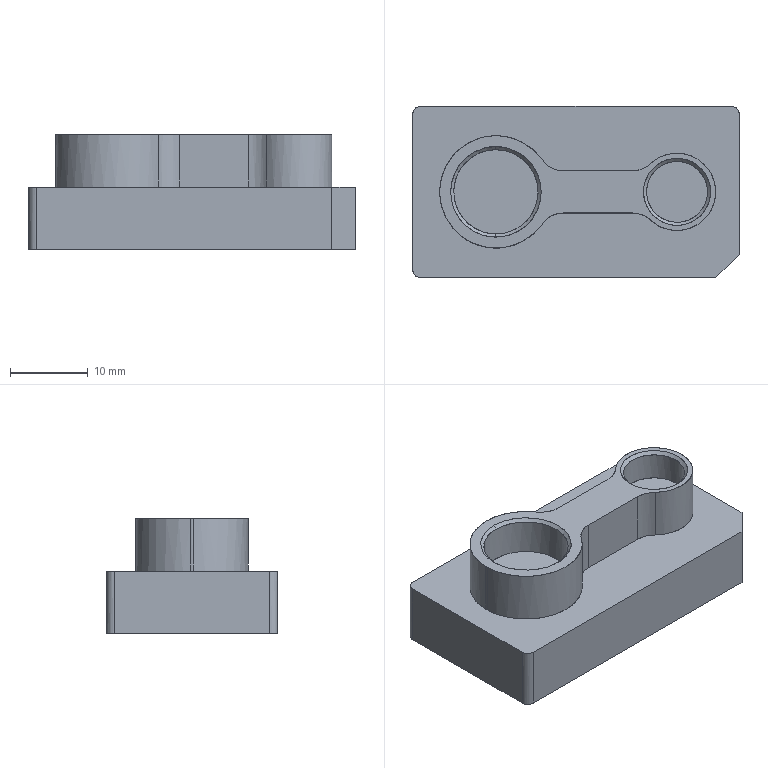NC program | PowerMill | posted by the shop | part box 42 x 22 x 14.721 mm
Lines 13163 to 14231 of 84704:
( TOOL ID   R1_1 )
( TOOL DIA. 2. TIP RAD 1. LENGTH 57. )
( Z = -1.104 )
T4 M6
T14
G91 G28 Z0
G0 G90 G54
M08
S18000 M3
X0 Y0 M8
G43 Z10.801 H4
X15.909 Y-2.486
Z.787
G1 Z-.413 F1200
X15.867 Y-2.527 Z-.416 F2000
X15.764 Y-2.63 Z-.42
X15.658 Y-2.737 Z-.421
X15.555 Y-2.84 Z-.418
X15.451 Y-2.943 Z-.411
X15.264 Y-3.088 Z-.412
X15.363 Y-2.989 Z-.424
X15.462 Y-2.89 Z-.433
X15.561 Y-2.791 Z-.439
X15.66 Y-2.692 Z-.441
X15.762 Y-2.59 Z-.44
X15.861 Y-2.491 Z-.435
X15.96 Y-2.392 Z-.427
X16.059 Y-2.293 Z-.416
X16.096 Y-2.256 Z-.411
X16.179 Y-2.13 Z-.413
X16.099 Y-2.211 Z-.426
X16.008 Y-2.301 Z-.439
X15.917 Y-2.392 Z-.45
X15.821 Y-2.489 Z-.458
X15.723 Y-2.587 Z-.463
X15.632 Y-2.678 Z-.464
X15.541 Y-2.769 Z-.461
X15.45 Y-2.86 Z-.455
X15.359 Y-2.95 Z-.446
X15.257 Y-3.053 Z-.433
X15.135 Y-3.174 Z-.414
X15.02 Y-3.247 Z-.415
X15.104 Y-3.163 Z-.431
X15.189 Y-3.078 Z-.447
X15.276 Y-2.991 Z-.461
X15.372 Y-2.895 Z-.473
X15.466 Y-2.801 Z-.482
X15.551 Y-2.717 Z-.486
X15.636 Y-2.632 Z-.488
X15.721 Y-2.547 Z-.486
X15.805 Y-2.462 Z-.481
X15.901 Y-2.366 Z-.472
X16.004 Y-2.263 Z-.459
X16.117 Y-2.15 Z-.44
X16.239 Y-2.028 Z-.416
X16.299 Y-1.926 Z-.418
X16.275 Y-1.949 Z-.423
X16.142 Y-2.083 Z-.452
X16.028 Y-2.197 Z-.474
X15.925 Y-2.3 Z-.491
X15.83 Y-2.394 Z-.503
X15.749 Y-2.476 Z-.51
X15.667 Y-2.558 Z-.514
X15.585 Y-2.64
X15.502 Y-2.723 Z-.511
X15.42 Y-2.804 Z-.505
X15.339 Y-2.886 Z-.496
X15.257 Y-2.967 Z-.485
X15.171 Y-3.053 Z-.47
X15.086 Y-3.139 Z-.453
X15. Y-3.225 Z-.434
X14.914 Y-3.31 Z-.415
X14.818 Y-3.365
X14.936 Y-3.246 Z-.445
X15.061 Y-3.121 Z-.475
X15.171 Y-3.011 Z-.498
X15.27 Y-2.912 Z-.516
X15.361 Y-2.821 Z-.529
X15.445 Y-2.737 Z-.537
X15.53 Y-2.652 Z-.542
X15.614 Y-2.568 Z-.543
X15.698 Y-2.484 Z-.54
X15.782 Y-2.401 Z-.533
X15.869 Y-2.313 Z-.523
X15.965 Y-2.218 Z-.507
X16.069 Y-2.113 Z-.486
X16.185 Y-1.998 Z-.46
X16.296 Y-1.886 Z-.432
X16.354 Y-1.828 Z-.417
X16.405 Y-1.735
X16.329 Y-1.811 Z-.438
X16.249 Y-1.891 Z-.46
X16.169 Y-1.971 Z-.482
X16.084 Y-2.056 Z-.504
X15.992 Y-2.148 Z-.525
X15.899 Y-2.241 Z-.543
X15.814 Y-2.326 Z-.557
X15.735 Y-2.404 Z-.566
X15.658 Y-2.482 Z-.571
X15.581 Y-2.559 Z-.573
X15.503 Y-2.637 Z-.572
X15.425 Y-2.714 Z-.567
X15.348 Y-2.792 Z-.56
X15.266 Y-2.873 Z-.548
X15.189 Y-2.951 Z-.534
X15.113 Y-3.027 Z-.517
X15.036 Y-3.104 Z-.499
X14.908 Y-3.232 Z-.465
X14.725 Y-3.415 Z-.414
X14.644 Y-3.453 Z-.415
X14.817 Y-3.28 Z-.467
X14.888 Y-3.209 Z-.489
X14.96 Y-3.138 Z-.51
X15.031 Y-3.066 Z-.53
X15.109 Y-2.988 Z-.55
X15.196 Y-2.902 Z-.569
X15.275 Y-2.822 Z-.583
X15.348 Y-2.75 Z-.592
X15.421 Y-2.677 Z-.599
X15.493 Y-2.604 Z-.602
X15.566 Y-2.531 Z-.603
X15.639 Y-2.458 Z-.601
X15.719 Y-2.378 Z-.595
X15.803 Y-2.295 Z-.585
X15.888 Y-2.209 Z-.571
X15.97 Y-2.127 Z-.554
X16.049 Y-2.048 Z-.534
X16.149 Y-1.948 Z-.507
X16.249 Y-1.848 Z-.477
X16.349 Y-1.749 Z-.446
X16.449 Y-1.649 Z-.416
Y-1.648
X16.485 Y-1.57
X16.449 Y-1.606 Z-.428
X16.389 Y-1.666 Z-.447
X16.329 Y-1.726 Z-.467
X16.27 Y-1.785 Z-.487
X16.21 Y-1.845 Z-.507
X16.15 Y-1.905 Z-.527
X16.09 Y-1.965 Z-.546
X16.023 Y-2.032 Z-.565
X15.959 Y-2.096 Z-.582
X15.898 Y-2.157 Z-.595
X15.837 Y-2.218 Z-.606
X15.776 Y-2.279 Z-.616
X15.702 Y-2.353 Z-.625
X15.618 Y-2.437 Z-.631
X15.533 Y-2.522 Z-.633
X15.449 Y-2.606 Z-.631
X15.364 Y-2.691 Z-.626
X15.279 Y-2.776 Z-.616
X15.199 Y-2.856 Z-.603
X15.117 Y-2.938 Z-.586
X15.029 Y-3.026 Z-.564
X14.933 Y-3.122 Z-.536
X14.855 Y-3.2 Z-.511
X14.71 Y-3.345 Z-.462
X14.565 Y-3.49 Z-.414
X14.492 Y-3.52 Z-.415
X14.704 Y-3.309 Z-.491
X14.796 Y-3.217 Z-.524
X14.891 Y-3.122 Z-.558
X14.982 Y-3.03 Z-.586
X15.07 Y-2.943 Z-.61
X15.155 Y-2.857 Z-.629
X15.238 Y-2.775 Z-.643
X15.321 Y-2.692 Z-.654
X15.404 Y-2.608 Z-.66
X15.489 Y-2.524 Z-.663
X15.573 Y-2.439 Z-.662
X15.659 Y-2.354 Z-.656
X15.744 Y-2.268 Z-.647
X15.83 Y-2.182 Z-.634
X15.916 Y-2.096 Z-.617
X15.972 Y-2.041 Z-.603
X16.027 Y-1.986 Z-.587
X16.082 Y-1.931 Z-.57
X16.137 Y-1.876 Z-.553
X16.192 Y-1.821 Z-.534
X16.246 Y-1.766 Z-.513
X16.426 Y-1.587 Z-.448
X16.519 Y-1.493 Z-.415
X16.549 Y-1.421 Z-.416
X16.467 Y-1.503 Z-.445
X16.349 Y-1.621 Z-.491
X16.246 Y-1.724 Z-.532
X16.166 Y-1.804 Z-.564
X16.086 Y-1.884 Z-.592
X16.003 Y-1.968 Z-.618
X15.916 Y-2.054 Z-.641
X15.834 Y-2.136 Z-.659
X15.752 Y-2.218 Z-.673
X15.67 Y-2.301 Z-.684
X15.585 Y-2.385 Z-.69
X15.501 Y-2.47 Z-.693
X15.416 Y-2.554 Z-.692
X15.332 Y-2.638 Z-.687
X15.248 Y-2.722 Z-.677
X15.164 Y-2.806 Z-.664
X15.08 Y-2.891 Z-.647
X14.994 Y-2.976 Z-.625
X14.909 Y-3.062 Z-.6
X14.822 Y-3.148 Z-.57
X14.74 Y-3.23 Z-.538
X14.635 Y-3.335 Z-.497
X14.529 Y-3.441 Z-.455
X14.423 Y-3.547 Z-.416
X14.353 Y-3.574
X14.441 Y-3.487 Z-.45
X14.538 Y-3.39 Z-.489
X14.653 Y-3.275 Z-.539
X14.741 Y-3.187 Z-.576
X14.829 Y-3.099 Z-.609
X14.916 Y-3.012 Z-.638
X15.004 Y-2.924 Z-.663
X15.087 Y-2.841 Z-.683
X15.171 Y-2.757 Z-.699
X15.255 Y-2.673 Z-.711
X15.339 Y-2.589 Z-.719
X15.422 Y-2.505 Z-.723
X15.506 Y-2.422
X15.589 Y-2.339 Z-.719
X15.671 Y-2.257 Z-.711
X15.754 Y-2.174 Z-.699
X15.834 Y-2.094 Z-.684
X15.899 Y-2.029 Z-.669
X15.964 Y-1.964 Z-.652
X16.028 Y-1.9 Z-.633
X16.092 Y-1.836 Z-.612
X16.156 Y-1.772 Z-.588
X16.219 Y-1.709 Z-.563
X16.282 Y-1.646 Z-.536
X16.345 Y-1.583 Z-.509
X16.408 Y-1.519 Z-.482
X16.472 Y-1.456 Z-.456
X16.535 Y-1.393 Z-.431
X16.578 Y-1.35 Z-.415
X16.601 Y-1.285 Z-.416
X16.577 Y-1.308 Z-.425
X16.477 Y-1.408 Z-.466
X16.428 Y-1.457 Z-.487
X16.379 Y-1.506 Z-.51
X16.313 Y-1.572 Z-.54
X16.264 Y-1.621 Z-.563
X16.215 Y-1.67 Z-.585
X16.166 Y-1.719 Z-.606
X16.095 Y-1.791 Z-.632
X16.019 Y-1.866 Z-.658
X15.934 Y-1.952 Z-.684
X15.857 Y-2.028 Z-.704
X15.781 Y-2.105 Z-.72
X15.701 Y-2.185 Z-.734
X15.618 Y-2.268 Z-.744
X15.534 Y-2.352 Z-.751
X15.453 Y-2.433 Z-.753
X15.372 Y-2.513 Z-.752
X15.289 Y-2.596 Z-.746
X15.206 Y-2.68 Z-.737
X15.122 Y-2.764 Z-.724
X15.037 Y-2.848 Z-.706
X14.953 Y-2.933 Z-.685
X14.868 Y-3.018 Z-.659
X14.782 Y-3.103 Z-.629
X14.699 Y-3.186 Z-.597
X14.623 Y-3.262 Z-.564
X14.529 Y-3.356 Z-.52
X14.442 Y-3.444 Z-.481
X14.352 Y-3.533 Z-.442
X14.288 Y-3.598 Z-.417
X14.223 Y-3.619
X14.282 Y-3.561 Z-.441
X14.34 Y-3.503 Z-.467
X14.398 Y-3.445 Z-.494
X14.456 Y-3.387 Z-.521
X14.529 Y-3.314 Z-.558
X14.602 Y-3.241 Z-.592
X14.689 Y-3.154 Z-.63
X14.779 Y-3.064 Z-.664
X14.87 Y-2.973 Z-.696
X14.948 Y-2.895 Z-.718
X15.028 Y-2.815 Z-.738
X15.112 Y-2.731 Z-.755
X15.196 Y-2.646 Z-.768
X15.278 Y-2.564 Z-.777
X15.358 Y-2.485 Z-.782
X15.437 Y-2.406 Z-.783
X15.519 Y-2.324 Z-.78
X15.602 Y-2.241 Z-.774
X15.685 Y-2.158 Z-.763
X15.769 Y-2.074 Z-.748
X15.854 Y-1.989 Z-.729
X15.939 Y-1.904 Z-.706
X16.025 Y-1.818 Z-.678
X16.111 Y-1.732 Z-.647
X16.188 Y-1.655 Z-.616
X16.256 Y-1.587 Z-.585
X16.337 Y-1.506 Z-.545
X16.398 Y-1.445 Z-.516
X16.462 Y-1.381 Z-.486
X16.52 Y-1.323 Z-.459
X16.586 Y-1.257 Z-.432
X16.621 Y-1.222 Z-.417
X16.641 Y-1.16
X16.598 Y-1.203 Z-.435
X16.504 Y-1.297 Z-.478
X16.414 Y-1.386 Z-.523
X16.325 Y-1.475 Z-.57
X16.244 Y-1.556 Z-.61
X16.156 Y-1.644 Z-.649
X16.068 Y-1.733 Z-.684
X15.981 Y-1.819 Z-.715
X15.896 Y-1.905 Z-.742
X15.811 Y-1.989 Z-.764
X15.727 Y-2.073 Z-.782
X15.644 Y-2.157 Z-.796
X15.561 Y-2.239 Z-.806
X15.48 Y-2.321 Z-.811
X15.399 Y-2.401 Z-.813
X15.317 Y-2.483 Z-.811
X15.235 Y-2.565 Z-.805
X15.153 Y-2.648 Z-.795
X15.07 Y-2.73 Z-.781
X14.987 Y-2.813 Z-.763
X14.903 Y-2.897 Z-.741
X14.819 Y-2.981 Z-.715
X14.735 Y-3.066 Z-.685
X14.656 Y-3.145 Z-.654
X14.583 Y-3.218 Z-.621
X14.508 Y-3.292 Z-.585
X14.442 Y-3.359 Z-.553
X14.372 Y-3.428 Z-.517
X14.297 Y-3.504 Z-.479
X14.24 Y-3.56 Z-.452
X14.161 Y-3.64 Z-.417
X14.099 Y-3.659
X14.163 Y-3.595 Z-.446
X14.225 Y-3.533 Z-.476
X14.288 Y-3.47 Z-.508
X14.354 Y-3.404 Z-.544
X14.418 Y-3.341 Z-.578
X14.481 Y-3.277 Z-.612
X14.57 Y-3.188 Z-.654
X14.652 Y-3.106 Z-.69
X14.741 Y-3.017 Z-.724
X14.827 Y-2.931 Z-.754
X14.91 Y-2.848 Z-.778
X14.993 Y-2.765 Z-.799
X15.077 Y-2.681 Z-.816
X15.16 Y-2.598 Z-.829
X15.243 Y-2.515 Z-.838
X15.322 Y-2.436 Z-.842
X15.4 Y-2.358 Z-.843
X15.482 Y-2.276 Z-.84
X15.565 Y-2.193 Z-.832
X15.648 Y-2.11 Z-.821
X15.728 Y-2.03 Z-.807
X15.798 Y-1.96 Z-.791
X15.872 Y-1.886 Z-.771
X15.966 Y-1.792 Z-.742
X15.999 Y-1.759 Z-.731
X16.032 Y-1.726 Z-.719
X16.065 Y-1.694 Z-.706
X16.097 Y-1.661 Z-.693
X16.14 Y-1.618 Z-.675
X16.173 Y-1.585 Z-.661
X16.205 Y-1.553 Z-.646
X16.237 Y-1.521 Z-.631
X16.269 Y-1.489 Z-.615
X16.354 Y-1.404 Z-.571
X16.436 Y-1.322 Z-.527
X16.508 Y-1.25 Z-.488
X16.568 Y-1.19 Z-.458
X16.635 Y-1.123 Z-.428
X16.66 Y-1.098 Z-.417
X16.68 Y-1.036 Z-.416
X16.64 Y-1.076 Z-.434
X16.58 Y-1.136 Z-.463
X16.524 Y-1.192 Z-.492
X16.46 Y-1.255 Z-.529
X16.392 Y-1.324 Z-.566
X16.295 Y-1.421 Z-.619
X16.228 Y-1.487 Z-.653
X16.139 Y-1.577 Z-.695
X16.051 Y-1.665 Z-.732
X15.964 Y-1.752 Z-.765
X15.879 Y-1.837 Z-.793
X15.795 Y-1.92 Z-.816
X15.712 Y-2.003 Z-.836
X15.63 Y-2.086 Z-.851
X15.548 Y-2.168 Z-.862
X15.466 Y-2.249 Z-.87
X15.385 Y-2.331 Z-.873
X15.304 Y-2.412 Z-.872
X15.223 Y-2.493 Z-.868
X15.142 Y-2.574 Z-.859
X15.06 Y-2.655 Z-.847
X14.978 Y-2.738 Z-.83
X14.894 Y-2.822 Z-.809
X14.809 Y-2.906 Z-.784
X14.723 Y-2.992 Z-.755
X14.637 Y-3.079 Z-.721
X14.561 Y-3.155 Z-.688
X14.477 Y-3.239 Z-.647
X14.371 Y-3.345 Z-.592
X14.328 Y-3.388 Z-.569
X14.277 Y-3.439 Z-.539
X14.234 Y-3.481 Z-.515
X14.156 Y-3.559 Z-.474
X14.092 Y-3.624 Z-.441
X14.039 Y-3.677 Z-.417
X13.978 Y-3.695 Z-.416
X14.014 Y-3.659 Z-.433
X14.05 Y-3.623 Z-.45
X14.086 Y-3.587 Z-.469
X14.159 Y-3.514 Z-.51
X14.242 Y-3.431 Z-.559
X14.325 Y-3.348 Z-.606
X14.393 Y-3.28 Z-.644
X14.462 Y-3.211 Z-.679
X14.551 Y-3.122 Z-.722
X14.638 Y-3.035 Z-.759
X14.723 Y-2.95 Z-.791
X14.808 Y-2.865 Z-.82
X14.892 Y-2.781 Z-.844
X14.975 Y-2.699 Z-.864
X15.057 Y-2.616 Z-.88
X15.139 Y-2.535 Z-.891
X15.22 Y-2.454 Z-.899
X15.3 Y-2.373 Z-.903
X15.355 Y-2.318
X15.41 Y-2.263 Z-.901
X15.465 Y-2.208 Z-.898
X15.52 Y-2.153 Z-.892
X15.575 Y-2.099 Z-.886
X15.629 Y-2.044 Z-.877
X15.715 Y-1.958 Z-.86
X15.801 Y-1.872 Z-.839
X15.886 Y-1.788 Z-.813
X15.969 Y-1.704 Z-.784
X16.053 Y-1.621 Z-.752
X16.141 Y-1.532 Z-.713
X16.233 Y-1.44 Z-.669
X16.292 Y-1.381 Z-.637
X16.351 Y-1.322 Z-.604
X16.41 Y-1.263 Z-.57
X16.459 Y-1.215 Z-.542
X16.518 Y-1.155 Z-.507
X16.566 Y-1.107 Z-.48
X16.622 Y-1.051 Z-.451
X16.679 Y-.994 Z-.423
X16.699 Y-.974 Z-.415
X16.713 Y-.917
X16.7 Y-.931 Z-.421
X16.643 Y-.987 Z-.448
X16.605 Y-1.026 Z-.469
X16.528 Y-1.103 Z-.513
X16.495 Y-1.136 Z-.533
X16.461 Y-1.17 Z-.553
X16.428 Y-1.203 Z-.574
X16.394 Y-1.236 Z-.594
X16.361 Y-1.27 Z-.615
X16.327 Y-1.304 Z-.634
X16.235 Y-1.396 Z-.685
X16.142 Y-1.489 Z-.731
X16.054 Y-1.577 Z-.771
X15.967 Y-1.664 Z-.806
X15.882 Y-1.749 Z-.837
X15.797 Y-1.833 Z-.863
X15.714 Y-1.917 Z-.885
X15.632 Y-1.999 Z-.903
X15.551 Y-2.08 Z-.916
X15.471 Y-2.16 Z-.926
X15.391 Y-2.24 Z-.931
X15.309 Y-2.321 Z-.933
X15.23 Y-2.4 Z-.931
X15.151 Y-2.48 Z-.925
X15.071 Y-2.56 Z-.915
X14.989 Y-2.642 Z-.901
X14.906 Y-2.724 Z-.882
X14.823 Y-2.808 Z-.86
X14.738 Y-2.892 Z-.833
X14.653 Y-2.978 Z-.802
X14.567 Y-3.064 Z-.766
X14.475 Y-3.155 Z-.724
X14.385 Y-3.246 Z-.679
X14.29 Y-3.341 Z-.626
X14.196 Y-3.435 Z-.57
X14.141 Y-3.49 Z-.536
X14.074 Y-3.556 Z-.496
X14.021 Y-3.61 Z-.466
X13.962 Y-3.668 Z-.436
X13.92 Y-3.711 Z-.416
X13.862 Y-3.726 Z-.415
X13.882 Y-3.707 Z-.424
X13.901 Y-3.687 Z-.434
X13.928 Y-3.661 Z-.447
X13.947 Y-3.641 Z-.458
X13.966 Y-3.622 Z-.468
X13.985 Y-3.603 Z-.479
X14.044 Y-3.545 Z-.515
X14.098 Y-3.49 Z-.549
X14.178 Y-3.41 Z-.599
X14.252 Y-3.336 Z-.644
X14.344 Y-3.244 Z-.696
X14.436 Y-3.152 Z-.744
X14.524 Y-3.064 Z-.785
X14.611 Y-2.977 Z-.823
X14.698 Y-2.89 Z-.856
X14.774 Y-2.814 Z-.881
X14.852 Y-2.736 Z-.903
X14.933 Y-2.655 Z-.923
X15.016 Y-2.572 Z-.94
X15.099 Y-2.49 Z-.952
X15.179 Y-2.409 Z-.96
X15.257 Y-2.331 Z-.964
X15.331 Y-2.257
X15.403 Y-2.185 Z-.961
X15.475 Y-2.113 Z-.954
X15.559 Y-2.03 Z-.942
X15.642 Y-1.946 Z-.926
X15.726 Y-1.862 Z-.906
X15.81 Y-1.778 Z-.882
X15.894 Y-1.694 Z-.854
X15.978 Y-1.61 Z-.822
X16.062 Y-1.526 Z-.786
X16.153 Y-1.435 Z-.743
X16.243 Y-1.345 Z-.697
X16.313 Y-1.276 Z-.657
X16.4 Y-1.188 Z-.604
X16.472 Y-1.116 Z-.56
X16.518 Y-1.07 Z-.531
X16.56 Y-1.028 Z-.504
X16.602 Y-.986 Z-.479
X16.667 Y-.922 Z-.444
X16.719 Y-.869 Z-.418
X16.725 Y-.864 Z-.415
X16.736 Y-.81 Z-.416
X16.731 Y-.815 Z-.419
X16.667 Y-.879 Z-.451
X16.603 Y-.943 Z-.488
X16.539 Y-1.007 Z-.529
X16.43 Y-1.116 Z-.6
X16.354 Y-1.192 Z-.648
X16.256 Y-1.289 Z-.705
X16.164 Y-1.382 Z-.755
X16.074 Y-1.472 Z-.799
X15.986 Y-1.559 Z-.839
X15.913 Y-1.633 Z-.868
X15.84 Y-1.706 Z-.895
X15.758 Y-1.788 Z-.921
X15.67 Y-1.876 Z-.945
X15.587 Y-1.959 Z-.964
X15.512 Y-2.034 Z-.978
X15.436 Y-2.11 Z-.989
X15.367 Y-2.179 Z-.996
X15.297 Y-2.249 Z-.999
X15.226 Y-2.32 Z-.998
X15.155 Y-2.391 Z-.994
X15.086 Y-2.46 Z-.986
X15.021 Y-2.525 Z-.976
X14.957 Y-2.589 Z-.964
X14.893 Y-2.653 Z-.949
X14.827 Y-2.719 Z-.932
X14.763 Y-2.783 Z-.913
X14.7 Y-2.846 Z-.893
X14.637 Y-2.909 Z-.87
X14.549 Y-2.997 Z-.834
X14.462 Y-3.084 Z-.795
X14.376 Y-3.17 Z-.752
X14.29 Y-3.256 Z-.706
X14.212 Y-3.334 Z-.66
X14.12 Y-3.426 Z-.602
X14.048 Y-3.498 Z-.556
X13.975 Y-3.571 Z-.508
X13.924 Y-3.622 Z-.477
X13.866 Y-3.68 Z-.444
X13.805 Y-3.741 Z-.414
X13.751 Y-3.753 Z-.413
X13.812 Y-3.691 Z-.446
X13.865 Y-3.638 Z-.475
X13.912 Y-3.591 Z-.505
X13.974 Y-3.529 Z-.547
X14.033 Y-3.471 Z-.586
X14.125 Y-3.378 Z-.647
X14.203 Y-3.301 Z-.695
X14.294 Y-3.21 Z-.747
X14.387 Y-3.116 Z-.796
X14.474 Y-3.03 Z-.839
X14.559 Y-2.944 Z-.876
X14.644 Y-2.86 Z-.909
X14.728 Y-2.776 Z-.938
X14.825 Y-2.679 Z-.968
X14.911 Y-2.592 Z-.992
X14.978 Y-2.526 Z-1.007
X15.042 Y-2.462 Z-1.019
X15.107 Y-2.397 Z-1.029
X15.174 Y-2.329 Z-1.035
X15.242 Y-2.262 Z-1.038
X15.308 Y-2.196 Z-1.036
X15.372 Y-2.131 Z-1.031
X15.436 Y-2.067 Z-1.023
X15.501 Y-2.003 Z-1.012
X15.567 Y-1.937 Z-.998
X15.633 Y-1.87 Z-.981
X15.699 Y-1.805 Z-.962
X15.764 Y-1.739 Z-.942
X15.847 Y-1.657 Z-.914
X15.932 Y-1.572 Z-.881
X16.018 Y-1.485 Z-.844
X16.107 Y-1.396 Z-.801
X16.199 Y-1.305 Z-.753
X16.292 Y-1.211 Z-.699
X16.372 Y-1.131 Z-.65
X16.462 Y-1.041 Z-.592
X16.586 Y-.918 Z-.509
X16.645 Y-.859 Z-.471
X16.705 Y-.798 Z-.437
X16.747 Y-.757 Z-.416
X16.758 Y-.703
X16.699 Y-.763 Z-.448
X16.638 Y-.823 Z-.483
X16.586 Y-.875 Z-.517
X16.557 Y-.904 Z-.538
X16.528 Y-.933 Z-.558
X16.499 Y-.962 Z-.578
X16.47 Y-.991 Z-.599
X16.44 Y-1.021 Z-.619
X16.411 Y-1.05 Z-.639
X16.322 Y-1.139 Z-.696
X16.253 Y-1.208 Z-.738
X16.184 Y-1.277 Z-.777
X16.102 Y-1.359 Z-.821
X16.019 Y-1.442 Z-.862
X15.982 Y-1.479 Z-.88
X15.945 Y-1.516 Z-.896
X15.908 Y-1.553 Z-.911
X15.871 Y-1.59 Z-.925
X15.83 Y-1.631 Z-.941
X15.768 Y-1.693 Z-.964
X15.723 Y-1.739 Z-.98
X15.685 Y-1.776 Z-.993
X15.648 Y-1.813 Z-1.006
X15.61 Y-1.851 Z-1.018
X15.572 Y-1.889 Z-1.029
X15.496 Y-1.965 Z-1.048
X15.424 Y-2.037 Z-1.063
X15.357 Y-2.104 Z-1.073
X15.292 Y-2.169 Z-1.079
X15.23 Y-2.231 Z-1.081
X15.167 Y-2.294 Z-1.079
X15.103 Y-2.359 Z-1.073
X15.035 Y-2.426 Z-1.063
X14.965 Y-2.496 Z-1.048
X14.89 Y-2.571 Z-1.029
X14.814 Y-2.647 Z-1.006
X14.729 Y-2.732 Z-.977
X14.644 Y-2.817 Z-.946
X14.559 Y-2.902 Z-.913
X14.474 Y-2.987 Z-.877
X14.388 Y-3.073 Z-.836
X14.3 Y-3.161 Z-.79
X14.211 Y-3.25 Z-.739
X14.109 Y-3.352 Z-.677
X14.028 Y-3.433 Z-.624
X13.947 Y-3.514 Z-.568
X13.887 Y-3.574 Z-.526
X13.827 Y-3.635 Z-.485
X13.763 Y-3.698 Z-.448
X13.697 Y-3.764 Z-.413
X13.645 Y-3.774 Z-.412
X13.698 Y-3.721 Z-.44
X13.756 Y-3.662 Z-.475
X13.818 Y-3.601 Z-.516
X13.89 Y-3.528 Z-.568
X13.971 Y-3.447 Z-.626
X14.037 Y-3.382 Z-.67
X14.137 Y-3.282 Z-.734
X14.23 Y-3.188 Z-.79
X14.32 Y-3.099 Z-.84
X14.386 Y-3.033 Z-.873
X14.425 Y-2.993 Z-.892
X14.465 Y-2.953 Z-.911
X14.505 Y-2.913 Z-.928
X14.547 Y-2.871 Z-.946
X14.6 Y-2.819 Z-.968
X14.675 Y-2.743 Z-.999
X14.735 Y-2.684 Z-1.023
X14.781 Y-2.637 Z-1.04
X14.822 Y-2.597 Z-1.055
X14.863 Y-2.556 Z-1.068
X14.904 Y-2.515 Z-1.081
X14.928 Y-2.491 Z-1.088
X14.774 Y-2.602
X14.772 Y-2.604
X14.685 Y-2.691 Z-1.051
X14.572 Y-2.804 Z-.999
X14.458 Y-2.919 Z-.946
X14.356 Y-3.02 Z-.897
X14.273 Y-3.103 Z-.854
X14.196 Y-3.18 Z-.81
X14.113 Y-3.263 Z-.76
X14.036 Y-3.34 Z-.71
X13.959 Y-3.417 Z-.657
X13.912 Y-3.464 Z-.626
X13.865 Y-3.511 Z-.592
X13.797 Y-3.58 Z-.54
X13.748 Y-3.628 Z-.505
X13.701 Y-3.675 Z-.474
X13.644 Y-3.732 Z-.439
X13.592 Y-3.784 Z-.411
X13.544 Y-3.79 Z-.412
X13.585 Y-3.749 Z-.435
X13.63 Y-3.704 Z-.462
X13.675 Y-3.659 Z-.491
X13.729 Y-3.605 Z-.53
X13.807 Y-3.526 Z-.59
X13.881 Y-3.452 Z-.644
X13.971 Y-3.362 Z-.708
X14.038 Y-3.296 Z-.752
X14.104 Y-3.23 Z-.794
X14.171 Y-3.163 Z-.835
X14.239 Y-3.095 Z-.874
X14.307 Y-3.026 Z-.91
X14.655 Y-2.679 Z-1.089
X14.554 Y-2.738 Z-1.091
X14.531 Y-2.76 Z-1.078
X14.445 Y-2.847 Z-1.027
X14.358 Y-2.934 Z-.978
X14.27 Y-3.021 Z-.93
X14.183 Y-3.108 Z-.882
X14.097 Y-3.194 Z-.83
X14.004 Y-3.287 Z-.771
X13.909 Y-3.382 Z-.705
X13.808 Y-3.483 Z-.632
X13.741 Y-3.55 Z-.581
X13.671 Y-3.621 Z-.526
X13.621 Y-3.67 Z-.489
X13.578 Y-3.713 Z-.461
X13.531 Y-3.761 Z-.432
X13.495 Y-3.796 Z-.413
X13.448 Y-3.801
X13.499 Y-3.75 Z-.442
X13.551 Y-3.698 Z-.476
X13.602 Y-3.647 Z-.513
X13.672 Y-3.577 Z-.568
X13.742 Y-3.507 Z-.623
X13.812 Y-3.437 Z-.676
X13.884 Y-3.365 Z-.728
X13.958 Y-3.291 Z-.781
X14.033 Y-3.216 Z-.83
X14.104 Y-3.145 Z-.874
X14.154 Y-3.095 Z-.904
X14.204 Y-3.044 Z-.933
X14.255 Y-2.994 Z-.963
X14.305 Y-2.944 Z-.993
X14.355 Y-2.893 Z-1.023
X14.403 Y-2.846 Z-1.054
X14.455 Y-2.794 Z-1.087
X14.463 Y-2.786 Z-1.092
X14.377 Y-2.83 Z-1.093
X14.354 Y-2.852 Z-1.076
X14.306 Y-2.9 Z-1.042
X14.257 Y-2.949 Z-1.01
X14.208 Y-2.998 Z-.978
X14.14 Y-3.066 Z-.936
X14.061 Y-3.146 Z-.888
X13.991 Y-3.216 Z-.843
X13.899 Y-3.307 Z-.78
X13.8 Y-3.407 Z-.708
X13.725 Y-3.481 Z-.651
X13.651 Y-3.555 Z-.592
X13.576 Y-3.63 Z-.533
X13.524 Y-3.683 Z-.492
X13.488 Y-3.718 Z-.467
X13.45 Y-3.757 Z-.443
X13.4 Y-3.806 Z-.413
X13.354 Y-3.81 Z-.414
X13.409 Y-3.755 Z-.446
X13.459 Y-3.705 Z-.48
X13.506 Y-3.658 Z-.516
X13.552 Y-3.612 Z-.554
X13.68 Y-3.484 Z-.658
X13.728 Y-3.436 Z-.695
X13.775 Y-3.389 Z-.731
X13.823 Y-3.341 Z-.766
X13.871 Y-3.293 Z-.801
X13.919 Y-3.245 Z-.835
X13.968 Y-3.196 Z-.868
X14.063 Y-3.101 Z-.929
X14.136 Y-3.028 Z-.976
X14.199 Y-2.965 Z-1.019
X14.264 Y-2.9 Z-1.067
X14.297 Y-2.867 Z-1.092
X14.221 Y-2.9 Z-1.093
X14.211 Y-2.911 Z-1.084
X14.168 Y-2.953 Z-1.049
X14.125 Y-2.997 Z-1.016
X14.081 Y-3.041 Z-.984
X14.036 Y-3.085 Z-.953
X13.968 Y-3.153 Z-.909
X13.911 Y-3.21 Z-.871
X13.854 Y-3.267 Z-.83
X13.789 Y-3.333 Z-.782
X13.724 Y-3.398 Z-.733
X13.659 Y-3.462 Z-.683
X13.615 Y-3.506 Z-.648
X13.563 Y-3.558 Z-.604
X13.506 Y-3.616 Z-.555
X13.462 Y-3.66 Z-.52
X13.4 Y-3.721 Z-.474
X13.351 Y-3.77 Z-.44
X13.308 Y-3.814 Z-.414
X13.262 Y-3.818
X13.31 Y-3.77 Z-.445
X13.351 Y-3.728 Z-.472
X13.382 Y-3.697 Z-.494
X13.412 Y-3.667 Z-.518
X13.441 Y-3.638 Z-.543
X13.471 Y-3.609 Z-.569
X13.5 Y-3.579 Z-.593
X13.592 Y-3.487 Z-.671
X13.659 Y-3.42 Z-.725
X13.727 Y-3.352 Z-.777
X13.795 Y-3.284 Z-.829
X13.864 Y-3.215 Z-.878
X13.934 Y-3.146 Z-.926
X14.003 Y-3.077 Z-.975
X14.051 Y-3.029 Z-1.01
X14.103 Y-2.976 Z-1.052
X14.149 Y-2.93 Z-1.092
X14.15
X14.082 Y-2.954 Z-1.094
X14.058 Y-2.979 Z-1.071
X14.027 Y-3.01 Z-1.043
X13.996 Y-3.041 Z-1.017
X13.964 Y-3.073 Z-.992
X13.918 Y-3.119 Z-.958
X13.847 Y-3.19 Z-.909
X13.801 Y-3.236 Z-.874
X13.747 Y-3.29 Z-.832
X13.64 Y-3.396 Z-.751
X13.566 Y-3.471 Z-.691
X13.492 Y-3.545 Z-.628
X13.438 Y-3.599 Z-.582
X13.383 Y-3.654 Z-.534
X13.338 Y-3.699 Z-.497
X13.303 Y-3.734 Z-.471
X13.267 Y-3.77 Z-.447
X13.216 Y-3.821 Z-.413
X13.171 Y-3.823
X13.186 Y-3.809 Z-.422
X13.2 Y-3.794 Z-.431
X13.219 Y-3.776 Z-.444
X13.243 Y-3.751 Z-.461
X13.259 Y-3.735 Z-.472
X13.273 Y-3.721 Z-.482
X13.287 Y-3.708 Z-.493
X13.332 Y-3.662 Z-.531
X13.393 Y-3.601 Z-.584
X13.445 Y-3.549 Z-.631
X13.567 Y-3.427 Z-.733
X13.663 Y-3.332 Z-.811
X13.73 Y-3.265 Z-.862
X13.831 Y-3.163 Z-.937
X13.876 Y-3.119 Z-.971
X13.931 Y-3.063 Z-1.015
X13.977 Y-3.017 Z-1.055
X14.017 Y-2.977 Z-1.094
X13.954 Y-2.998
X13.911 Y-3.041 Z-1.052
X13.862 Y-3.09 Z-1.008
X13.814 Y-3.138 Z-.969
X13.739 Y-3.213 Z-.91
X13.663 Y-3.289 Z-.852
X13.588 Y-3.364 Z-.792
X13.513 Y-3.439 Z-.731
X13.44 Y-3.512 Z-.668
X13.328 Y-3.624 Z-.569
X13.283 Y-3.669 Z-.528
X13.237 Y-3.715 Z-.49
X13.185 Y-3.767 Z-.452
X13.126 Y-3.825 Z-.413
X13.082 Y-3.827 Z-.412
X13.14 Y-3.769 Z-.452
X13.197 Y-3.713 Z-.495
X13.252 Y-3.657 Z-.542
X13.306 Y-3.603 Z-.591
X13.369 Y-3.54 Z-.647
X13.432 Y-3.477 Z-.704
X13.48 Y-3.429 Z-.745
X13.528 Y-3.381 Z-.785
X13.577 Y-3.332 Z-.824
X13.626 Y-3.284 Z-.863
X13.675 Y-3.235 Z-.902
X13.724 Y-3.186 Z-.941
X13.772 Y-3.138 Z-.981
X13.83 Y-3.08 Z-1.032
X13.886 Y-3.024 Z-1.087
X13.893 Y-3.017 Z-1.094
X13.833 Y-3.034
X13.809 Y-3.058 Z-1.067
X13.774 Y-3.093 Z-1.032
X13.735 Y-3.132 Z-.997
X13.704 Y-3.163 Z-.969
X13.661 Y-3.206 Z-.933
X13.599 Y-3.268 Z-.884
X13.549 Y-3.318 Z-.844
X13.435 Y-3.432 Z-.748
X13.331 Y-3.536 Z-.657
X13.279 Y-3.588 Z-.608
X13.217 Y-3.651 Z-.549
X13.171 Y-3.697 Z-.509
X13.132 Y-3.735 Z-.478
X13.093 Y-3.774 Z-.45
X13.038 Y-3.829 Z-.412
X12.995 Y-3.83 Z-.411
X13.053 Y-3.772 Z-.451
X13.104 Y-3.72 Z-.491
X13.151 Y-3.674 Z-.531
X13.195 Y-3.63 Z-.573
X13.287 Y-3.538 Z-.658
X13.38 Y-3.444 Z-.742
X13.445 Y-3.379 Z-.799
X13.515 Y-3.31 Z-.857
X13.548 Y-3.277 Z-.885
X13.579 Y-3.246 Z-.91
X13.614 Y-3.211 Z-.938
X13.644 Y-3.181 Z-.964
X13.67 Y-3.155 Z-.987
X13.695 Y-3.129 Z-1.01
X13.721 Y-3.104 Z-1.035
X13.75 Y-3.075 Z-1.064
X13.773 Y-3.051 Z-1.091
X13.775 Y-3.049 Z-1.094
X13.719 Y-3.063
X13.7 Y-3.083 Z-1.072
X13.654 Y-3.128 Z-1.023
X13.607 Y-3.175 Z-.978
X13.559 Y-3.223 Z-.936
X13.467 Y-3.315 Z-.86
X13.381 Y-3.401 Z-.785
X13.299 Y-3.483 Z-.712
X13.219 Y-3.563 Z-.637
X13.109 Y-3.673 Z-.534
X13.078 Y-3.704 Z-.504
X13.045 Y-3.737 Z-.477
X13.006 Y-3.776 Z-.448
X12.952 Y-3.831 Z-.411
X12.909 Z-.41
X12.947 Y-3.792 Z-.436
X12.974 Y-3.765 Z-.455
X13.001 Y-3.739 Z-.477
X13.052 Y-3.688 Z-.522
X13.118 Y-3.622 Z-.584
X13.215 Y-3.524 Z-.676
X13.314 Y-3.426 Z-.768
X13.394 Y-3.346 Z-.839
X13.475 Y-3.265 Z-.908
X13.535 Y-3.204 Z-.961
X13.58 Y-3.16 Z-1.002
X13.623 Y-3.117 Z-1.047
X13.664 Y-3.076 Z-1.094
X13.61 Y-3.087 Z-1.093
X13.572 Y-3.125 Z-1.048
X13.53 Y-3.167 Z-1.004
X13.485 Y-3.213 Z-.961
X13.399 Y-3.299 Z-.884
X13.303 Y-3.395 Z-.8
X13.208 Y-3.489 Z-.713
X13.114 Y-3.583 Z-.623
X13.068 Y-3.629 Z-.578
X13.006 Y-3.692 Z-.519
X12.956 Y-3.741 Z-.475
X12.931 Y-3.767 Z-.454
X12.904 Y-3.794 Z-.435
X12.866 Y-3.832 Z-.409
X12.824 Y-3.831
X12.866 Y-3.789 Z-.437
X12.898 Y-3.757 Z-.461
X12.927 Y-3.728 Z-.485
X12.971 Y-3.684 Z-.525
X13.022 Y-3.633 Z-.574
X13.126 Y-3.529 Z-.675
X13.23 Y-3.425 Z-.775
X13.321 Y-3.334 Z-.858
X13.4 Y-3.255 Z-.928
X13.445 Y-3.21 Z-.969
X13.491 Y-3.164 Z-1.016
X13.538 Y-3.116 Z-1.07
X13.558 Y-3.096 Z-1.094
X13.507 Y-3.105
X13.501 Y-3.112 Z-1.086
X13.469 Y-3.144 Z-1.046
X13.433 Y-3.18 Z-1.006
X13.402 Y-3.211 Z-.974
X13.37 Y-3.243 Z-.944
X13.337 Y-3.275 Z-.915
X13.305 Y-3.308 Z-.886
X13.245 Y-3.367 Z-.831
X13.152 Y-3.461 Z-.744
X13.069 Y-3.543 Z-.664
X12.949 Y-3.663 Z-.544
X12.912 Y-3.701 Z-.508
X12.873 Y-3.739 Z-.473
X12.831 Y-3.782 Z-.441
X12.785 Y-3.828 Z-.409
X12.745 Y-3.825 Z-.41
X12.779 Y-3.791 Z-.434
X12.808 Y-3.763 Z-.454
X12.835 Y-3.735 Z-.476
X12.872 Y-3.698 Z-.51
X12.922 Y-3.648 Z-.559
X12.975 Y-3.595 Z-.611
X13.062 Y-3.509 Z-.698
X13.131 Y-3.439 Z-.766
X13.251 Y-3.319 Z-.879
X13.315 Y-3.255 Z-.937
X13.348 Y-3.222 Z-.969
X13.377 Y-3.193 Z-.998
X13.403 Y-3.167 Z-1.027
X13.433 Y-3.137 Z-1.062
X13.457 Y-3.113 Z-1.094
X13.407 Y-3.12
X13.393 Y-3.134 Z-1.074
X13.367 Y-3.161 Z-1.04
X13.339 Y-3.189 Z-1.008
X13.31 Y-3.217 Z-.978
X13.281 Y-3.247 Z-.949
X13.25 Y-3.277 Z-.921
X13.142 Y-3.386 Z-.819
X13.069 Y-3.459 Z-.748
X12.906 Y-3.622 Z-.584
X12.881 Y-3.647 Z-.559
X12.856 Y-3.672 Z-.533
X12.83 Y-3.697 Z-.508
X12.804 Y-3.723 Z-.485
X12.778 Y-3.75 Z-.462
X12.745 Y-3.782 Z-.438
X12.706 Y-3.822 Z-.41
X12.667 Y-3.818
X12.713 Y-3.772 Z-.443
X12.756 Y-3.729 Z-.478
X12.796 Y-3.689 Z-.515
X12.835 Y-3.65 Z-.554
X12.962 Y-3.523 Z-.683
X13.09 Y-3.395 Z-.81
X13.134 Y-3.351 Z-.854
X13.175 Y-3.31 Z-.892
X13.216 Y-3.269 Z-.93
X13.247 Y-3.238 Z-.961
X13.294 Y-3.191 Z-1.012
X13.328 Y-3.158 Z-1.052
X13.355 Y-3.13 Z-1.088
X13.359 Y-3.126 Z-1.094
X13.312 Y-3.131 Z-1.093
X13.282 Y-3.161 Z-1.054
X13.259 Y-3.183 Z-1.025
X13.234 Y-3.209 Z-.997
X13.191 Y-3.252 Z-.952
X13.121 Y-3.322 Z-.883
X13.01 Y-3.433 Z-.775
X12.94 Y-3.503 Z-.704
X12.88 Y-3.562 Z-.643
X12.817 Y-3.626 Z-.577
X12.764 Y-3.678 Z-.523
X12.722 Y-3.721 Z-.482
X12.699 Y-3.744 Z-.462
X12.676 Y-3.767 Z-.444
X12.652 Y-3.79 Z-.427